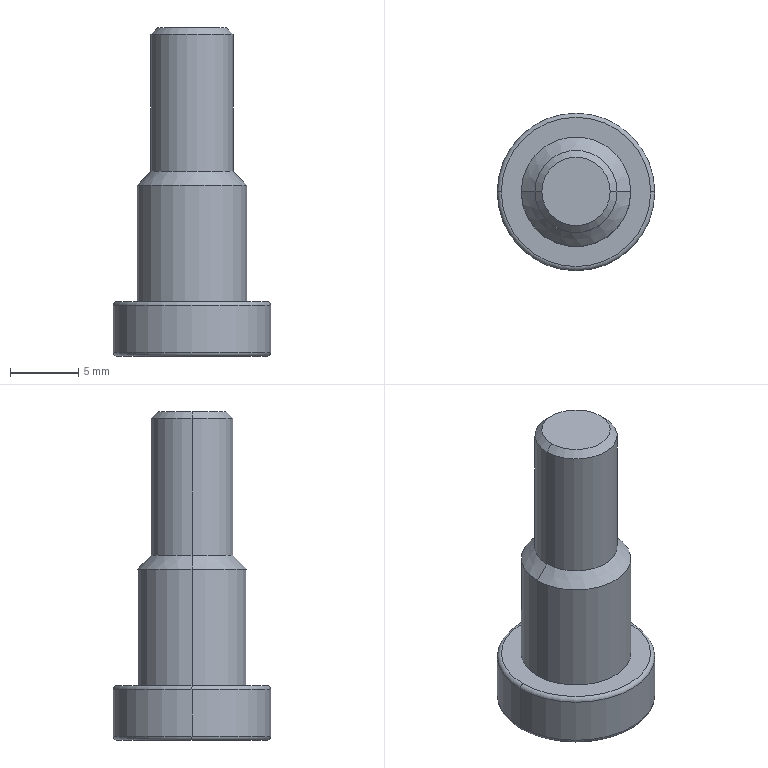Part | 1 solid | 26 faces | box 11.5 x 11.5 x 24 mm | volume 1109 mm3 | plane 10 | cone 6 | cylinder 6 | torus 4 | commonest cylinder face diameters 6 x2 8 x2 11.5 x2
STEP:
#1=CARTESIAN_POINT('',(-5.45,0.,0.));
#2=VERTEX_POINT('',#1);
#3=CARTESIAN_POINT('',(5.45,0.,0.));
#4=VERTEX_POINT('',#3);
#5=CARTESIAN_POINT('',(0.,0.,0.));
#6=DIRECTION('',(0.,0.,-1.));
#7=DIRECTION('',(1.,0.,0.));
#8=AXIS2_PLACEMENT_3D('',#5,#6,#7);
#9=CIRCLE('',#8,5.45);
#10=EDGE_CURVE('',#2,#4,#9,.T.);
#11=ORIENTED_EDGE('',*,*,#10,.F.);
#12=CARTESIAN_POINT('',(-5.75,0.,0.3));
#13=VERTEX_POINT('',#12);
#14=CARTESIAN_POINT('',(-5.45,0.,0.3));
#15=DIRECTION('',(0.,1.,0.));
#16=DIRECTION('',(-1.,0.,0.));
#17=AXIS2_PLACEMENT_3D('',#14,#15,#16);
#18=CIRCLE('',#17,0.3);
#19=EDGE_CURVE('',#2,#13,#18,.T.);
#20=ORIENTED_EDGE('',*,*,#19,.T.);
#21=CARTESIAN_POINT('',(5.75,0.,0.3));
#22=VERTEX_POINT('',#21);
#23=CARTESIAN_POINT('',(0.,0.,0.3));
#24=DIRECTION('',(0.,0.,1.));
#25=DIRECTION('',(1.,0.,0.));
#26=AXIS2_PLACEMENT_3D('',#23,#24,#25);
#27=CIRCLE('',#26,5.75);
#28=EDGE_CURVE('',#22,#13,#27,.T.);
#29=ORIENTED_EDGE('',*,*,#28,.F.);
#30=CARTESIAN_POINT('',(5.45,0.,0.3));
#31=DIRECTION('',(0.,-1.,0.));
#32=DIRECTION('',(0.,0.,-1.));
#33=AXIS2_PLACEMENT_3D('',#30,#31,#32);
#34=CIRCLE('',#33,0.3);
#35=EDGE_CURVE('',#4,#22,#34,.T.);
#36=ORIENTED_EDGE('',*,*,#35,.F.);
#37=EDGE_LOOP('',(#11,#20,#29,#36));
#38=FACE_OUTER_BOUND('',#37,.T.);
#39=CARTESIAN_POINT('',(0.,0.,0.3));
#40=DIRECTION('',(0.,0.,1.));
#41=DIRECTION('',(1.,0.,0.));
#42=AXIS2_PLACEMENT_3D('',#39,#40,#41);
#43=TOROIDAL_SURFACE('',#42,5.45,0.3);
#44=ADVANCED_FACE('',(#38),#43,.T.);
#45=CARTESIAN_POINT('',(-5.75,0.,3.7));
#46=VERTEX_POINT('',#45);
#47=CARTESIAN_POINT('',(5.75,0.,3.7));
#48=VERTEX_POINT('',#47);
#49=CARTESIAN_POINT('',(0.,0.,3.7));
#50=DIRECTION('',(0.,0.,-1.));
#51=DIRECTION('',(1.,0.,0.));
#52=AXIS2_PLACEMENT_3D('',#49,#50,#51);
#53=CIRCLE('',#52,5.75);
#54=EDGE_CURVE('',#46,#48,#53,.T.);
#55=ORIENTED_EDGE('',*,*,#54,.F.);
#56=CARTESIAN_POINT('',(-5.45,0.,4.));
#57=VERTEX_POINT('',#56);
#58=CARTESIAN_POINT('',(-5.45,0.,3.7));
#59=DIRECTION('',(0.,1.,0.));
#60=DIRECTION('',(-1.,0.,0.));
#61=AXIS2_PLACEMENT_3D('',#58,#59,#60);
#62=CIRCLE('',#61,0.3);
#63=EDGE_CURVE('',#46,#57,#62,.T.);
#64=ORIENTED_EDGE('',*,*,#63,.T.);
#65=CARTESIAN_POINT('',(5.45,0.,4.));
#66=VERTEX_POINT('',#65);
#67=CARTESIAN_POINT('',(0.,0.,4.));
#68=DIRECTION('',(0.,0.,1.));
#69=DIRECTION('',(1.,0.,0.));
#70=AXIS2_PLACEMENT_3D('',#67,#68,#69);
#71=CIRCLE('',#70,5.45);
#72=EDGE_CURVE('',#66,#57,#71,.T.);
#73=ORIENTED_EDGE('',*,*,#72,.F.);
#74=CARTESIAN_POINT('',(5.45,0.,3.7));
#75=DIRECTION('',(0.,-1.,0.));
#76=DIRECTION('',(0.,0.,-1.));
#77=AXIS2_PLACEMENT_3D('',#74,#75,#76);
#78=CIRCLE('',#77,0.3);
#79=EDGE_CURVE('',#48,#66,#78,.T.);
#80=ORIENTED_EDGE('',*,*,#79,.F.);
#81=EDGE_LOOP('',(#55,#64,#73,#80));
#82=FACE_OUTER_BOUND('',#81,.T.);
#83=CARTESIAN_POINT('',(0.,0.,3.7));
#84=DIRECTION('',(0.,0.,1.));
#85=DIRECTION('',(1.,0.,0.));
#86=AXIS2_PLACEMENT_3D('',#83,#84,#85);
#87=TOROIDAL_SURFACE('',#86,5.45,0.3);
#88=ADVANCED_FACE('',(#82),#87,.T.);
#89=CARTESIAN_POINT('',(2.887,0.,0.01325));
#90=VERTEX_POINT('',#89);
#91=CARTESIAN_POINT('',(1.443,-2.5,0.01325));
#92=VERTEX_POINT('',#91);
#93=CARTESIAN_POINT('',(2.887,0.,0.01325));
#94=CARTESIAN_POINT('',(2.826,-0.1053,0.07405));
#95=CARTESIAN_POINT('',(2.737,-0.2595,0.1543));
#96=CARTESIAN_POINT('',(2.637,-0.4329,0.2287));
#97=CARTESIAN_POINT('',(2.588,-0.518,0.2612));
#98=CARTESIAN_POINT('',(2.567,-0.5541,0.274));
#99=CARTESIAN_POINT('',(2.553,-0.5781,0.2824));
#100=CARTESIAN_POINT('',(2.547,-0.5883,0.2859));
#101=CARTESIAN_POINT('',(2.413,-0.8207,0.3629));
#102=CARTESIAN_POINT('',(2.289,-1.035,0.3994));
#103=CARTESIAN_POINT('',(2.107,-1.35,0.4003));
#104=CARTESIAN_POINT('',(2.015,-1.51,0.3871));
#105=CARTESIAN_POINT('',(1.906,-1.699,0.3481));
#106=CARTESIAN_POINT('',(1.851,-1.794,0.3226));
#107=CARTESIAN_POINT('',(1.827,-1.835,0.3104));
#108=CARTESIAN_POINT('',(1.812,-1.862,0.302));
#109=CARTESIAN_POINT('',(1.803,-1.878,0.2971));
#110=CARTESIAN_POINT('',(1.684,-2.083,0.2301));
#111=CARTESIAN_POINT('',(1.567,-2.286,0.1368));
#112=CARTESIAN_POINT('',(1.443,-2.5,0.01325));
#113=B_SPLINE_CURVE_WITH_KNOTS('',3,(#93,#94,#95,#96,#97,#98,#99,#100,#101,#102,#103,#104,#105,#106,#107,#108,#109,#110,#111,#112),.UNSPECIFIED.,.F.,.F.,(4,1,1,1,2,2,2,1,1,1,2,2,4),(0.,0.125,0.1875,0.2187,0.2344,0.25,0.5,0.625,0.6875,0.7187,0.7344,0.75,1.),.UNSPECIFIED.);
#114=EDGE_CURVE('',#90,#92,#113,.T.);
#115=ORIENTED_EDGE('',*,*,#114,.F.);
#116=CARTESIAN_POINT('',(2.9,0.,0.));
#117=VERTEX_POINT('',#116);
#118=CARTESIAN_POINT('',(2.4,0.,0.5));
#119=DIRECTION('',(0.7071,0.,-0.7071));
#120=VECTOR('',#119,1000.);
#121=LINE('',#118,#120);
#122=EDGE_CURVE('',#90,#117,#121,.T.);
#123=ORIENTED_EDGE('',*,*,#122,.T.);
#124=CARTESIAN_POINT('',(-2.9,0.,0.));
#125=VERTEX_POINT('',#124);
#126=CARTESIAN_POINT('',(0.,0.,0.));
#127=DIRECTION('',(0.,0.,1.));
#128=DIRECTION('',(1.,0.,0.));
#129=AXIS2_PLACEMENT_3D('',#126,#127,#128);
#130=CIRCLE('',#129,2.9);
#131=EDGE_CURVE('',#125,#117,#130,.T.);
#132=ORIENTED_EDGE('',*,*,#131,.F.);
#133=CARTESIAN_POINT('',(-2.887,0.,0.01325));
#134=VERTEX_POINT('',#133);
#135=CARTESIAN_POINT('',(-2.4,0.,0.5));
#136=DIRECTION('',(-0.7071,0.,-0.7071));
#137=VECTOR('',#136,1000.);
#138=LINE('',#135,#137);
#139=EDGE_CURVE('',#134,#125,#138,.T.);
#140=ORIENTED_EDGE('',*,*,#139,.F.);
#141=CARTESIAN_POINT('',(-1.443,-2.5,0.01325));
#142=VERTEX_POINT('',#141);
#143=CARTESIAN_POINT('',(-1.443,-2.5,0.01325));
#144=CARTESIAN_POINT('',(-1.504,-2.395,0.07405));
#145=CARTESIAN_POINT('',(-1.593,-2.24,0.1543));
#146=CARTESIAN_POINT('',(-1.693,-2.067,0.2287));
#147=CARTESIAN_POINT('',(-1.742,-1.982,0.2612));
#148=CARTESIAN_POINT('',(-1.763,-1.946,0.274));
#149=CARTESIAN_POINT('',(-1.777,-1.922,0.2824));
#150=CARTESIAN_POINT('',(-1.783,-1.912,0.2859));
#151=CARTESIAN_POINT('',(-1.917,-1.679,0.3629));
#152=CARTESIAN_POINT('',(-2.041,-1.465,0.3994));
#153=CARTESIAN_POINT('',(-2.223,-1.15,0.4003));
#154=CARTESIAN_POINT('',(-2.315,-0.9904,0.3871));
#155=CARTESIAN_POINT('',(-2.424,-0.8014,0.3481));
#156=CARTESIAN_POINT('',(-2.479,-0.7061,0.3226));
#157=CARTESIAN_POINT('',(-2.503,-0.6651,0.3104));
#158=CARTESIAN_POINT('',(-2.519,-0.6377,0.302));
#159=CARTESIAN_POINT('',(-2.527,-0.6224,0.2971));
#160=CARTESIAN_POINT('',(-2.646,-0.4174,0.2301));
#161=CARTESIAN_POINT('',(-2.763,-0.214,0.1368));
#162=CARTESIAN_POINT('',(-2.887,0.,0.01325));
#163=B_SPLINE_CURVE_WITH_KNOTS('',3,(#143,#144,#145,#146,#147,#148,#149,#150,#151,#152,#153,#154,#155,#156,#157,#158,#159,#160,#161,#162),.UNSPECIFIED.,.F.,.F.,(4,1,1,1,2,2,2,1,1,1,2,2,4),(0.,0.125,0.1875,0.2188,0.2344,0.25,0.5,0.625,0.6875,0.7187,0.7344,0.75,1.),.UNSPECIFIED.);
#164=EDGE_CURVE('',#142,#134,#163,.T.);
#165=ORIENTED_EDGE('',*,*,#164,.F.);
#166=CARTESIAN_POINT('',(1.443,-2.5,0.01325));
#167=CARTESIAN_POINT('',(1.321,-2.5,0.0745));
#168=CARTESIAN_POINT('',(1.142,-2.5,0.1553));
#169=CARTESIAN_POINT('',(0.9399,-2.5,0.23));
#170=CARTESIAN_POINT('',(0.841,-2.5,0.2626));
#171=CARTESIAN_POINT('',(0.799,-2.5,0.2754));
#172=CARTESIAN_POINT('',(0.7711,-2.5,0.2838));
#173=CARTESIAN_POINT('',(0.7591,-2.5,0.2873));
#174=CARTESIAN_POINT('',(0.4909,-2.5,0.3638));
#175=CARTESIAN_POINT('',(0.2428,-2.5,0.3999));
#176=CARTESIAN_POINT('',(-0.1205,-2.5,0.4001));
#177=CARTESIAN_POINT('',(-0.3043,-2.5,0.3866));
#178=CARTESIAN_POINT('',(-0.5223,-2.5,0.3472));
#179=CARTESIAN_POINT('',(-0.6323,-2.5,0.3215));
#180=CARTESIAN_POINT('',(-0.6796,-2.5,0.3093));
#181=CARTESIAN_POINT('',(-0.7112,-2.5,0.3008));
#182=CARTESIAN_POINT('',(-0.729,-2.5,0.2959));
#183=CARTESIAN_POINT('',(-0.9643,-2.5,0.2289));
#184=CARTESIAN_POINT('',(-1.198,-2.5,0.136));
#185=CARTESIAN_POINT('',(-1.443,-2.5,0.01325));
#186=B_SPLINE_CURVE_WITH_KNOTS('',3,(#166,#167,#168,#169,#170,#171,#172,#173,#174,#175,#176,#177,#178,#179,#180,#181,#182,#183,#184,#185),.UNSPECIFIED.,.F.,.F.,(4,1,1,1,2,2,2,1,1,1,2,2,4),(0.,0.125,0.1875,0.2187,0.2344,0.25,0.5,0.625,0.6875,0.7187,0.7344,0.75,1.),.UNSPECIFIED.);
#187=EDGE_CURVE('',#92,#142,#186,.T.);
#188=ORIENTED_EDGE('',*,*,#187,.F.);
#189=EDGE_LOOP('',(#115,#123,#132,#140,#165,#188));
#190=FACE_OUTER_BOUND('',#189,.T.);
#191=CARTESIAN_POINT('',(0.,0.,0.5));
#192=DIRECTION('',(0.,0.,-1.));
#193=DIRECTION('',(-1.,0.,0.));
#194=AXIS2_PLACEMENT_3D('',#191,#192,#193);
#195=CONICAL_SURFACE('',#194,2.4,0.7854);
#196=ADVANCED_FACE('',(#190),#195,.F.);
#197=CARTESIAN_POINT('',(2.5,0.,24.));
#198=VERTEX_POINT('',#197);
#199=CARTESIAN_POINT('',(-2.5,0.,24.));
#200=VERTEX_POINT('',#199);
#201=CARTESIAN_POINT('',(0.,0.,24.));
#202=DIRECTION('',(0.,0.,1.));
#203=DIRECTION('',(1.,0.,0.));
#204=AXIS2_PLACEMENT_3D('',#201,#202,#203);
#205=CIRCLE('',#204,2.5);
#206=EDGE_CURVE('',#198,#200,#205,.T.);
#207=ORIENTED_EDGE('',*,*,#206,.F.);
#208=CARTESIAN_POINT('',(3.,0.,23.5));
#209=VERTEX_POINT('',#208);
#210=CARTESIAN_POINT('',(2.5,0.,24.));
#211=DIRECTION('',(0.7071,0.,-0.7071));
#212=VECTOR('',#211,1000.);
#213=LINE('',#210,#212);
#214=EDGE_CURVE('',#198,#209,#213,.T.);
#215=ORIENTED_EDGE('',*,*,#214,.T.);
#216=CARTESIAN_POINT('',(-3.,0.,23.5));
#217=VERTEX_POINT('',#216);
#218=CARTESIAN_POINT('',(0.,0.,23.5));
#219=DIRECTION('',(0.,0.,-1.));
#220=DIRECTION('',(1.,0.,0.));
#221=AXIS2_PLACEMENT_3D('',#218,#219,#220);
#222=CIRCLE('',#221,3.);
#223=EDGE_CURVE('',#217,#209,#222,.T.);
#224=ORIENTED_EDGE('',*,*,#223,.F.);
#225=CARTESIAN_POINT('',(-2.5,0.,24.));
#226=DIRECTION('',(-0.7071,0.,-0.7071));
#227=VECTOR('',#226,1000.);
#228=LINE('',#225,#227);
#229=EDGE_CURVE('',#200,#217,#228,.T.);
#230=ORIENTED_EDGE('',*,*,#229,.F.);
#231=EDGE_LOOP('',(#207,#215,#224,#230));
#232=FACE_OUTER_BOUND('',#231,.T.);
#233=CARTESIAN_POINT('',(0.,0.,24.));
#234=DIRECTION('',(0.,0.,-1.));
#235=DIRECTION('',(-1.,0.,0.));
#236=AXIS2_PLACEMENT_3D('',#233,#234,#235);
#237=CONICAL_SURFACE('',#236,2.5,0.7854);
#238=ADVANCED_FACE('',(#232),#237,.T.);
#239=CARTESIAN_POINT('',(3.,0.,13.5));
#240=VERTEX_POINT('',#239);
#241=CARTESIAN_POINT('',(-3.,0.,13.5));
#242=VERTEX_POINT('',#241);
#243=CARTESIAN_POINT('',(0.,0.,13.5));
#244=DIRECTION('',(0.,0.,1.));
#245=DIRECTION('',(1.,0.,0.));
#246=AXIS2_PLACEMENT_3D('',#243,#244,#245);
#247=CIRCLE('',#246,3.);
#248=EDGE_CURVE('',#240,#242,#247,.T.);
#249=ORIENTED_EDGE('',*,*,#248,.F.);
#250=CARTESIAN_POINT('',(4.,0.,12.5));
#251=VERTEX_POINT('',#250);
#252=CARTESIAN_POINT('',(3.,0.,13.5));
#253=DIRECTION('',(0.7071,0.,-0.7071));
#254=VECTOR('',#253,1000.);
#255=LINE('',#252,#254);
#256=EDGE_CURVE('',#240,#251,#255,.T.);
#257=ORIENTED_EDGE('',*,*,#256,.T.);
#258=CARTESIAN_POINT('',(-4.,0.,12.5));
#259=VERTEX_POINT('',#258);
#260=CARTESIAN_POINT('',(0.,0.,12.5));
#261=DIRECTION('',(0.,0.,-1.));
#262=DIRECTION('',(1.,0.,0.));
#263=AXIS2_PLACEMENT_3D('',#260,#261,#262);
#264=CIRCLE('',#263,4.);
#265=EDGE_CURVE('',#259,#251,#264,.T.);
#266=ORIENTED_EDGE('',*,*,#265,.F.);
#267=CARTESIAN_POINT('',(-3.,0.,13.5));
#268=DIRECTION('',(-0.7071,0.,-0.7071));
#269=VECTOR('',#268,1000.);
#270=LINE('',#267,#269);
#271=EDGE_CURVE('',#242,#259,#270,.T.);
#272=ORIENTED_EDGE('',*,*,#271,.F.);
#273=EDGE_LOOP('',(#249,#257,#266,#272));
#274=FACE_OUTER_BOUND('',#273,.T.);
#275=CARTESIAN_POINT('',(0.,0.,13.5));
#276=DIRECTION('',(0.,0.,-1.));
#277=DIRECTION('',(-1.,0.,0.));
#278=AXIS2_PLACEMENT_3D('',#275,#276,#277);
#279=CONICAL_SURFACE('',#278,3.,0.7854);
#280=ADVANCED_FACE('',(#274),#279,.T.);
#281=ORIENTED_EDGE('',*,*,#223,.T.);
#282=CARTESIAN_POINT('',(3.,0.,24.));
#283=DIRECTION('',(0.,0.,-1.));
#284=VECTOR('',#283,1000.);
#285=LINE('',#282,#284);
#286=EDGE_CURVE('',#209,#240,#285,.T.);
#287=ORIENTED_EDGE('',*,*,#286,.T.);
#288=ORIENTED_EDGE('',*,*,#248,.T.);
#289=CARTESIAN_POINT('',(-3.,0.,24.));
#290=DIRECTION('',(0.,0.,-1.));
#291=VECTOR('',#290,1000.);
#292=LINE('',#289,#291);
#293=EDGE_CURVE('',#217,#242,#292,.T.);
#294=ORIENTED_EDGE('',*,*,#293,.F.);
#295=EDGE_LOOP('',(#281,#287,#288,#294));
#296=FACE_OUTER_BOUND('',#295,.T.);
#297=CARTESIAN_POINT('',(0.,0.,24.));
#298=DIRECTION('',(0.,0.,-1.));
#299=DIRECTION('',(-1.,0.,0.));
#300=AXIS2_PLACEMENT_3D('',#297,#298,#299);
#301=CYLINDRICAL_SURFACE('',#300,3.);
#302=ADVANCED_FACE('',(#296),#301,.T.);
#303=ORIENTED_EDGE('',*,*,#265,.T.);
#304=CARTESIAN_POINT('',(4.,0.,4.));
#305=VERTEX_POINT('',#304);
#306=CARTESIAN_POINT('',(4.,0.,13.5));
#307=DIRECTION('',(0.,0.,-1.));
#308=VECTOR('',#307,1000.);
#309=LINE('',#306,#308);
#310=EDGE_CURVE('',#251,#305,#309,.T.);
#311=ORIENTED_EDGE('',*,*,#310,.T.);
#312=CARTESIAN_POINT('',(-4.,0.,4.));
#313=VERTEX_POINT('',#312);
#314=CARTESIAN_POINT('',(0.,0.,4.));
#315=DIRECTION('',(0.,0.,1.));
#316=DIRECTION('',(1.,0.,0.));
#317=AXIS2_PLACEMENT_3D('',#314,#315,#316);
#318=CIRCLE('',#317,4.);
#319=EDGE_CURVE('',#305,#313,#318,.T.);
#320=ORIENTED_EDGE('',*,*,#319,.T.);
#321=CARTESIAN_POINT('',(-4.,0.,13.5));
#322=DIRECTION('',(0.,0.,-1.));
#323=VECTOR('',#322,1000.);
#324=LINE('',#321,#323);
#325=EDGE_CURVE('',#259,#313,#324,.T.);
#326=ORIENTED_EDGE('',*,*,#325,.F.);
#327=EDGE_LOOP('',(#303,#311,#320,#326));
#328=FACE_OUTER_BOUND('',#327,.T.);
#329=CARTESIAN_POINT('',(0.,0.,13.5));
#330=DIRECTION('',(0.,0.,-1.));
#331=DIRECTION('',(-1.,0.,0.));
#332=AXIS2_PLACEMENT_3D('',#329,#330,#331);
#333=CYLINDRICAL_SURFACE('',#332,4.);
#334=ADVANCED_FACE('',(#328),#333,.T.);
#335=ORIENTED_EDGE('',*,*,#54,.T.);
#336=CARTESIAN_POINT('',(5.75,0.,4.));
#337=DIRECTION('',(0.,0.,-1.));
#338=VECTOR('',#337,1000.);
#339=LINE('',#336,#338);
#340=EDGE_CURVE('',#48,#22,#339,.T.);
#341=ORIENTED_EDGE('',*,*,#340,.T.);
#342=ORIENTED_EDGE('',*,*,#28,.T.);
#343=CARTESIAN_POINT('',(-5.75,0.,4.));
#344=DIRECTION('',(0.,0.,-1.));
#345=VECTOR('',#344,1000.);
#346=LINE('',#343,#345);
#347=EDGE_CURVE('',#46,#13,#346,.T.);
#348=ORIENTED_EDGE('',*,*,#347,.F.);
#349=EDGE_LOOP('',(#335,#341,#342,#348));
#350=FACE_OUTER_BOUND('',#349,.T.);
#351=CARTESIAN_POINT('',(0.,0.,4.));
#352=DIRECTION('',(0.,0.,-1.));
#353=DIRECTION('',(-1.,0.,0.));
#354=AXIS2_PLACEMENT_3D('',#351,#352,#353);
#355=CYLINDRICAL_SURFACE('',#354,5.75);
#356=ADVANCED_FACE('',(#350),#355,.T.);
#357=ORIENTED_EDGE('',*,*,#340,.F.);
#358=CARTESIAN_POINT('',(0.,0.,3.7));
#359=DIRECTION('',(0.,0.,-1.));
#360=DIRECTION('',(1.,0.,0.));
#361=AXIS2_PLACEMENT_3D('',#358,#359,#360);
#362=CIRCLE('',#361,5.75);
#363=EDGE_CURVE('',#48,#46,#362,.T.);
#364=ORIENTED_EDGE('',*,*,#363,.T.);
#365=ORIENTED_EDGE('',*,*,#347,.T.);
#366=CARTESIAN_POINT('',(0.,0.,0.3));
#367=DIRECTION('',(0.,0.,1.));
#368=DIRECTION('',(1.,0.,0.));
#369=AXIS2_PLACEMENT_3D('',#366,#367,#368);
#370=CIRCLE('',#369,5.75);
#371=EDGE_CURVE('',#13,#22,#370,.T.);
#372=ORIENTED_EDGE('',*,*,#371,.T.);
#373=EDGE_LOOP('',(#357,#364,#365,#372));
#374=FACE_OUTER_BOUND('',#373,.T.);
#375=CARTESIAN_POINT('',(0.,0.,4.));
#376=DIRECTION('',(0.,0.,-1.));
#377=DIRECTION('',(-1.,0.,0.));
#378=AXIS2_PLACEMENT_3D('',#375,#376,#377);
#379=CYLINDRICAL_SURFACE('',#378,5.75);
#380=ADVANCED_FACE('',(#374),#379,.T.);
#381=ORIENTED_EDGE('',*,*,#72,.T.);
#382=CARTESIAN_POINT('',(0.,0.,4.));
#383=DIRECTION('',(0.,0.,1.));
#384=DIRECTION('',(1.,0.,0.));
#385=AXIS2_PLACEMENT_3D('',#382,#383,#384);
#386=CIRCLE('',#385,5.45);
#387=EDGE_CURVE('',#57,#66,#386,.T.);
#388=ORIENTED_EDGE('',*,*,#387,.T.);
#389=EDGE_LOOP('',(#381,#388));
#390=FACE_OUTER_BOUND('',#389,.T.);
#391=CARTESIAN_POINT('',(0.,0.,4.));
#392=DIRECTION('',(0.,0.,1.));
#393=DIRECTION('',(1.,0.,0.));
#394=AXIS2_PLACEMENT_3D('',#391,#392,#393);
#395=CIRCLE('',#394,4.);
#396=EDGE_CURVE('',#313,#305,#395,.T.);
#397=ORIENTED_EDGE('',*,*,#396,.F.);
#398=ORIENTED_EDGE('',*,*,#319,.F.);
#399=EDGE_LOOP('',(#397,#398));
#400=FACE_BOUND('',#399,.T.);
#401=CARTESIAN_POINT('',(0.,0.,4.));
#402=DIRECTION('',(0.,0.,1.));
#403=DIRECTION('',(1.,0.,0.));
#404=AXIS2_PLACEMENT_3D('',#401,#402,#403);
#405=PLANE('',#404);
#406=ADVANCED_FACE('',(#390,#400),#405,.T.);
#407=CARTESIAN_POINT('',(0.,0.,0.));
#408=DIRECTION('',(0.,0.,-1.));
#409=DIRECTION('',(1.,0.,0.));
#410=AXIS2_PLACEMENT_3D('',#407,#408,#409);
#411=CIRCLE('',#410,5.45);
#412=EDGE_CURVE('',#4,#2,#411,.T.);
#413=ORIENTED_EDGE('',*,*,#412,.T.);
#414=ORIENTED_EDGE('',*,*,#10,.T.);
#415=EDGE_LOOP('',(#413,#414));
#416=FACE_OUTER_BOUND('',#415,.T.);
#417=ORIENTED_EDGE('',*,*,#131,.T.);
#418=CARTESIAN_POINT('',(0.,0.,0.));
#419=DIRECTION('',(0.,0.,1.));
#420=DIRECTION('',(1.,0.,0.));
#421=AXIS2_PLACEMENT_3D('',#418,#419,#420);
#422=CIRCLE('',#421,2.9);
#423=EDGE_CURVE('',#117,#125,#422,.T.);
#424=ORIENTED_EDGE('',*,*,#423,.T.);
#425=EDGE_LOOP('',(#417,#424));
#426=FACE_BOUND('',#425,.T.);
#427=CARTESIAN_POINT('',(0.,0.,0.));
#428=DIRECTION('',(0.,0.,1.));
#429=DIRECTION('',(1.,0.,0.));
#430=AXIS2_PLACEMENT_3D('',#427,#428,#429);
#431=PLANE('',#430);
#432=ADVANCED_FACE('',(#416,#426),#431,.F.);
#433=ORIENTED_EDGE('',*,*,#310,.F.);
#434=CARTESIAN_POINT('',(0.,0.,12.5));
#435=DIRECTION('',(0.,0.,-1.));
#436=DIRECTION('',(1.,0.,0.));
#437=AXIS2_PLACEMENT_3D('',#434,#435,#436);
#438=CIRCLE('',#437,4.);
#439=EDGE_CURVE('',#251,#259,#438,.T.);
#440=ORIENTED_EDGE('',*,*,#439,.T.);
#441=ORIENTED_EDGE('',*,*,#325,.T.);
#442=ORIENTED_EDGE('',*,*,#396,.T.);
#443=EDGE_LOOP('',(#433,#440,#441,#442));
#444=FACE_OUTER_BOUND('',#443,.T.);
#445=CARTESIAN_POINT('',(0.,0.,13.5));
#446=DIRECTION('',(0.,0.,-1.));
#447=DIRECTION('',(-1.,0.,0.));
#448=AXIS2_PLACEMENT_3D('',#445,#446,#447);
#449=CYLINDRICAL_SURFACE('',#448,4.);
#450=ADVANCED_FACE('',(#444),#449,.T.);
#451=ORIENTED_EDGE('',*,*,#286,.F.);
#452=CARTESIAN_POINT('',(0.,0.,23.5));
#453=DIRECTION('',(0.,0.,-1.));
#454=DIRECTION('',(1.,0.,0.));
#455=AXIS2_PLACEMENT_3D('',#452,#453,#454);
#456=CIRCLE('',#455,3.);
#457=EDGE_CURVE('',#209,#217,#456,.T.);
#458=ORIENTED_EDGE('',*,*,#457,.T.);
#459=ORIENTED_EDGE('',*,*,#293,.T.);
#460=CARTESIAN_POINT('',(0.,0.,13.5));
#461=DIRECTION('',(0.,0.,1.));
#462=DIRECTION('',(1.,0.,0.));
#463=AXIS2_PLACEMENT_3D('',#460,#461,#462);
#464=CIRCLE('',#463,3.);
#465=EDGE_CURVE('',#242,#240,#464,.T.);
#466=ORIENTED_EDGE('',*,*,#465,.T.);
#467=EDGE_LOOP('',(#451,#458,#459,#466));
#468=FACE_OUTER_BOUND('',#467,.T.);
#469=CARTESIAN_POINT('',(0.,0.,24.));
#470=DIRECTION('',(0.,0.,-1.));
#471=DIRECTION('',(-1.,0.,0.));
#472=AXIS2_PLACEMENT_3D('',#469,#470,#471);
#473=CYLINDRICAL_SURFACE('',#472,3.);
#474=ADVANCED_FACE('',(#468),#473,.T.);
#475=CARTESIAN_POINT('',(0.,0.,24.));
#476=DIRECTION('',(0.,0.,1.));
#477=DIRECTION('',(1.,0.,0.));
#478=AXIS2_PLACEMENT_3D('',#475,#476,#477);
#479=CIRCLE('',#478,2.5);
#480=EDGE_CURVE('',#200,#198,#479,.T.);
#481=ORIENTED_EDGE('',*,*,#480,.T.);
#482=ORIENTED_EDGE('',*,*,#206,.T.);
#483=EDGE_LOOP('',(#481,#482));
#484=FACE_OUTER_BOUND('',#483,.T.);
#485=CARTESIAN_POINT('',(0.,0.,24.));
#486=DIRECTION('',(0.,0.,1.));
#487=DIRECTION('',(1.,0.,0.));
#488=AXIS2_PLACEMENT_3D('',#485,#486,#487);
#489=PLANE('',#488);
#490=ADVANCED_FACE('',(#484),#489,.T.);
#491=ORIENTED_EDGE('',*,*,#256,.F.);
#492=ORIENTED_EDGE('',*,*,#465,.F.);
#493=ORIENTED_EDGE('',*,*,#271,.T.);
#494=ORIENTED_EDGE('',*,*,#439,.F.);
#495=EDGE_LOOP('',(#491,#492,#493,#494));
#496=FACE_OUTER_BOUND('',#495,.T.);
#497=CARTESIAN_POINT('',(0.,0.,13.5));
#498=DIRECTION('',(0.,0.,-1.));
#499=DIRECTION('',(-1.,0.,0.));
#500=AXIS2_PLACEMENT_3D('',#497,#498,#499);
#501=CONICAL_SURFACE('',#500,3.,0.7854);
#502=ADVANCED_FACE('',(#496),#501,.T.);
#503=ORIENTED_EDGE('',*,*,#214,.F.);
#504=ORIENTED_EDGE('',*,*,#480,.F.);
#505=ORIENTED_EDGE('',*,*,#229,.T.);
#506=ORIENTED_EDGE('',*,*,#457,.F.);
#507=EDGE_LOOP('',(#503,#504,#505,#506));
#508=FACE_OUTER_BOUND('',#507,.T.);
#509=CARTESIAN_POINT('',(0.,0.,24.));
#510=DIRECTION('',(0.,0.,-1.));
#511=DIRECTION('',(-1.,0.,0.));
#512=AXIS2_PLACEMENT_3D('',#509,#510,#511);
#513=CONICAL_SURFACE('',#512,2.5,0.7854);
#514=ADVANCED_FACE('',(#508),#513,.T.);
#515=ORIENTED_EDGE('',*,*,#122,.F.);
#516=CARTESIAN_POINT('',(1.443,2.5,0.01325));
#517=VERTEX_POINT('',#516);
#518=CARTESIAN_POINT('',(1.443,2.5,0.01325));
#519=CARTESIAN_POINT('',(1.504,2.395,0.07405));
#520=CARTESIAN_POINT('',(1.593,2.24,0.1543));
#521=CARTESIAN_POINT('',(1.693,2.067,0.2287));
#522=CARTESIAN_POINT('',(1.742,1.982,0.2612));
#523=CARTESIAN_POINT('',(1.763,1.946,0.274));
#524=CARTESIAN_POINT('',(1.777,1.922,0.2824));
#525=CARTESIAN_POINT('',(1.783,1.912,0.2859));
#526=CARTESIAN_POINT('',(1.917,1.679,0.3629));
#527=CARTESIAN_POINT('',(2.041,1.465,0.3994));
#528=CARTESIAN_POINT('',(2.223,1.15,0.4003));
#529=CARTESIAN_POINT('',(2.315,0.9904,0.3871));
#530=CARTESIAN_POINT('',(2.424,0.8014,0.3481));
#531=CARTESIAN_POINT('',(2.479,0.7061,0.3226));
#532=CARTESIAN_POINT('',(2.503,0.6651,0.3104));
#533=CARTESIAN_POINT('',(2.519,0.6377,0.302));
#534=CARTESIAN_POINT('',(2.527,0.6224,0.2971));
#535=CARTESIAN_POINT('',(2.646,0.4174,0.2301));
#536=CARTESIAN_POINT('',(2.763,0.214,0.1368));
#537=CARTESIAN_POINT('',(2.887,0.,0.01325));
#538=B_SPLINE_CURVE_WITH_KNOTS('',3,(#518,#519,#520,#521,#522,#523,#524,#525,#526,#527,#528,#529,#530,#531,#532,#533,#534,#535,#536,#537),.UNSPECIFIED.,.F.,.F.,(4,1,1,1,2,2,2,1,1,1,2,2,4),(0.,0.125,0.1875,0.2187,0.2344,0.25,0.5,0.625,0.6875,0.7188,0.7344,0.75,1.),.UNSPECIFIED.);
#539=EDGE_CURVE('',#517,#90,#538,.T.);
#540=ORIENTED_EDGE('',*,*,#539,.F.);
#541=CARTESIAN_POINT('',(-1.443,2.5,0.01325));
#542=VERTEX_POINT('',#541);
#543=CARTESIAN_POINT('',(-1.443,2.5,0.01325));
#544=CARTESIAN_POINT('',(-1.321,2.5,0.07454));
#545=CARTESIAN_POINT('',(-1.141,2.5,0.1553));
#546=CARTESIAN_POINT('',(-0.9395,2.5,0.2301));
#547=CARTESIAN_POINT('',(-0.8406,2.5,0.2627));
#548=CARTESIAN_POINT('',(-0.7986,2.5,0.2756));
#549=CARTESIAN_POINT('',(-0.7706,2.5,0.2839));
#550=CARTESIAN_POINT('',(-0.7587,2.5,0.2875));
#551=CARTESIAN_POINT('',(-0.4902,2.5,0.364));
#552=CARTESIAN_POINT('',(-0.2414,2.5,0.4));
#553=CARTESIAN_POINT('',(0.1216,2.5,0.4));
#554=CARTESIAN_POINT('',(0.3052,2.5,0.3865));
#555=CARTESIAN_POINT('',(0.523,2.5,0.347));
#556=CARTESIAN_POINT('',(0.6329,2.5,0.3214));
#557=CARTESIAN_POINT('',(0.6801,2.5,0.3092));
#558=CARTESIAN_POINT('',(0.7117,2.5,0.3007));
#559=CARTESIAN_POINT('',(0.7295,2.5,0.2958));
#560=CARTESIAN_POINT('',(0.9647,2.5,0.2288));
#561=CARTESIAN_POINT('',(1.198,2.5,0.1359));
#562=CARTESIAN_POINT('',(1.443,2.5,0.01325));
#563=B_SPLINE_CURVE_WITH_KNOTS('',3,(#543,#544,#545,#546,#547,#548,#549,#550,#551,#552,#553,#554,#555,#556,#557,#558,#559,#560,#561,#562),.UNSPECIFIED.,.F.,.F.,(4,1,1,1,2,2,2,1,1,1,2,2,4),(0.,0.125,0.1875,0.2188,0.2344,0.25,0.5,0.625,0.6875,0.7188,0.7344,0.75,1.),.UNSPECIFIED.);
#564=EDGE_CURVE('',#542,#517,#563,.T.);
#565=ORIENTED_EDGE('',*,*,#564,.F.);
#566=CARTESIAN_POINT('',(-2.887,0.,0.01325));
#567=CARTESIAN_POINT('',(-2.826,0.1053,0.07405));
#568=CARTESIAN_POINT('',(-2.737,0.2595,0.1543));
#569=CARTESIAN_POINT('',(-2.637,0.4329,0.2287));
#570=CARTESIAN_POINT('',(-2.588,0.518,0.2612));
#571=CARTESIAN_POINT('',(-2.567,0.5541,0.274));
#572=CARTESIAN_POINT('',(-2.553,0.5781,0.2824));
#573=CARTESIAN_POINT('',(-2.547,0.5883,0.2859));
#574=CARTESIAN_POINT('',(-2.413,0.8207,0.3629));
#575=CARTESIAN_POINT('',(-2.289,1.035,0.3994));
#576=CARTESIAN_POINT('',(-2.107,1.35,0.4003));
#577=CARTESIAN_POINT('',(-2.015,1.51,0.3871));
#578=CARTESIAN_POINT('',(-1.906,1.699,0.3481));
#579=CARTESIAN_POINT('',(-1.851,1.794,0.3226));
#580=CARTESIAN_POINT('',(-1.827,1.835,0.3104));
#581=CARTESIAN_POINT('',(-1.812,1.862,0.302));
#582=CARTESIAN_POINT('',(-1.803,1.878,0.2971));
#583=CARTESIAN_POINT('',(-1.684,2.083,0.2301));
#584=CARTESIAN_POINT('',(-1.567,2.286,0.1368));
#585=CARTESIAN_POINT('',(-1.443,2.5,0.01325));
#586=B_SPLINE_CURVE_WITH_KNOTS('',3,(#566,#567,#568,#569,#570,#571,#572,#573,#574,#575,#576,#577,#578,#579,#580,#581,#582,#583,#584,#585),.UNSPECIFIED.,.F.,.F.,(4,1,1,1,2,2,2,1,1,1,2,2,4),(0.,0.125,0.1875,0.2187,0.2344,0.25,0.5,0.625,0.6875,0.7187,0.7344,0.75,1.),.UNSPECIFIED.);
#587=EDGE_CURVE('',#134,#542,#586,.T.);
#588=ORIENTED_EDGE('',*,*,#587,.F.);
#589=ORIENTED_EDGE('',*,*,#139,.T.);
#590=ORIENTED_EDGE('',*,*,#423,.F.);
#591=EDGE_LOOP('',(#515,#540,#565,#588,#589,#590));
#592=FACE_OUTER_BOUND('',#591,.T.);
#593=CARTESIAN_POINT('',(0.,0.,0.5));
#594=DIRECTION('',(0.,0.,-1.));
#595=DIRECTION('',(-1.,0.,0.));
#596=AXIS2_PLACEMENT_3D('',#593,#594,#595);
#597=CONICAL_SURFACE('',#596,2.4,0.7854);
#598=ADVANCED_FACE('',(#592),#597,.F.);
#599=ORIENTED_EDGE('',*,*,#587,.T.);
#600=CARTESIAN_POINT('',(-1.443,2.5,3.));
#601=VERTEX_POINT('',#600);
#602=CARTESIAN_POINT('',(-1.443,2.5,3.));
#603=DIRECTION('',(0.,0.,-1.));
#604=VECTOR('',#603,1000.);
#605=LINE('',#602,#604);
#606=EDGE_CURVE('',#601,#542,#605,.T.);
#607=ORIENTED_EDGE('',*,*,#606,.F.);
#608=CARTESIAN_POINT('',(-2.887,0.,3.));
#609=VERTEX_POINT('',#608);
#610=CARTESIAN_POINT('',(-2.887,0.,3.));
#611=DIRECTION('',(0.5,0.866,0.));
#612=VECTOR('',#611,1000.);
#613=LINE('',#610,#612);
#614=EDGE_CURVE('',#609,#601,#613,.T.);
#615=ORIENTED_EDGE('',*,*,#614,.F.);
#616=CARTESIAN_POINT('',(-2.887,0.,3.));
#617=DIRECTION('',(0.,0.,-1.));
#618=VECTOR('',#617,1000.);
#619=LINE('',#616,#618);
#620=EDGE_CURVE('',#609,#134,#619,.T.);
#621=ORIENTED_EDGE('',*,*,#620,.T.);
#622=EDGE_LOOP('',(#599,#607,#615,#621));
#623=FACE_OUTER_BOUND('',#622,.T.);
#624=CARTESIAN_POINT('',(-2.887,0.,3.));
#625=DIRECTION('',(-0.866,0.5,0.));
#626=DIRECTION('',(0.,0.,1.));
#627=AXIS2_PLACEMENT_3D('',#624,#625,#626);
#628=PLANE('',#627);
#629=ADVANCED_FACE('',(#623),#628,.F.);
#630=ORIENTED_EDGE('',*,*,#164,.T.);
#631=ORIENTED_EDGE('',*,*,#620,.F.);
#632=CARTESIAN_POINT('',(-1.443,-2.5,3.));
#633=VERTEX_POINT('',#632);
#634=CARTESIAN_POINT('',(-1.443,-2.5,3.));
#635=DIRECTION('',(-0.5,0.866,0.));
#636=VECTOR('',#635,1000.);
#637=LINE('',#634,#636);
#638=EDGE_CURVE('',#633,#609,#637,.T.);
#639=ORIENTED_EDGE('',*,*,#638,.F.);
#640=CARTESIAN_POINT('',(-1.443,-2.5,3.));
#641=DIRECTION('',(0.,0.,-1.));
#642=VECTOR('',#641,1000.);
#643=LINE('',#640,#642);
#644=EDGE_CURVE('',#633,#142,#643,.T.);
#645=ORIENTED_EDGE('',*,*,#644,.T.);
#646=EDGE_LOOP('',(#630,#631,#639,#645));
#647=FACE_OUTER_BOUND('',#646,.T.);
#648=CARTESIAN_POINT('',(-1.443,-2.5,3.));
#649=DIRECTION('',(-0.866,-0.5,0.));
#650=DIRECTION('',(-0.5,0.866,0.));
#651=AXIS2_PLACEMENT_3D('',#648,#649,#650);
#652=PLANE('',#651);
#653=ADVANCED_FACE('',(#647),#652,.F.);
#654=ORIENTED_EDGE('',*,*,#187,.T.);
#655=ORIENTED_EDGE('',*,*,#644,.F.);
#656=CARTESIAN_POINT('',(1.443,-2.5,3.));
#657=VERTEX_POINT('',#656);
#658=CARTESIAN_POINT('',(1.443,-2.5,3.));
#659=DIRECTION('',(-1.,0.,0.));
#660=VECTOR('',#659,1000.);
#661=LINE('',#658,#660);
#662=EDGE_CURVE('',#657,#633,#661,.T.);
#663=ORIENTED_EDGE('',*,*,#662,.F.);
#664=CARTESIAN_POINT('',(1.443,-2.5,3.));
#665=DIRECTION('',(0.,0.,-1.));
#666=VECTOR('',#665,1000.);
#667=LINE('',#664,#666);
#668=EDGE_CURVE('',#657,#92,#667,.T.);
#669=ORIENTED_EDGE('',*,*,#668,.T.);
#670=EDGE_LOOP('',(#654,#655,#663,#669));
#671=FACE_OUTER_BOUND('',#670,.T.);
#672=CARTESIAN_POINT('',(1.443,-2.5,3.));
#673=DIRECTION('',(0.,-1.,0.));
#674=DIRECTION('',(0.,0.,-1.));
#675=AXIS2_PLACEMENT_3D('',#672,#673,#674);
#676=PLANE('',#675);
#677=ADVANCED_FACE('',(#671),#676,.F.);
#678=ORIENTED_EDGE('',*,*,#114,.T.);
#679=ORIENTED_EDGE('',*,*,#668,.F.);
#680=CARTESIAN_POINT('',(2.887,0.,3.));
#681=VERTEX_POINT('',#680);
#682=CARTESIAN_POINT('',(2.887,0.,3.));
#683=DIRECTION('',(-0.5,-0.866,0.));
#684=VECTOR('',#683,1000.);
#685=LINE('',#682,#684);
#686=EDGE_CURVE('',#681,#657,#685,.T.);
#687=ORIENTED_EDGE('',*,*,#686,.F.);
#688=CARTESIAN_POINT('',(2.887,0.,3.));
#689=DIRECTION('',(0.,0.,-1.));
#690=VECTOR('',#689,1000.);
#691=LINE('',#688,#690);
#692=EDGE_CURVE('',#681,#90,#691,.T.);
#693=ORIENTED_EDGE('',*,*,#692,.T.);
#694=EDGE_LOOP('',(#678,#679,#687,#693));
#695=FACE_OUTER_BOUND('',#694,.T.);
#696=CARTESIAN_POINT('',(2.887,0.,3.));
#697=DIRECTION('',(0.866,-0.5,0.));
#698=DIRECTION('',(0.,0.,-1.));
#699=AXIS2_PLACEMENT_3D('',#696,#697,#698);
#700=PLANE('',#699);
#701=ADVANCED_FACE('',(#695),#700,.F.);
#702=ORIENTED_EDGE('',*,*,#539,.T.);
#703=ORIENTED_EDGE('',*,*,#692,.F.);
#704=CARTESIAN_POINT('',(1.443,2.5,3.));
#705=VERTEX_POINT('',#704);
#706=CARTESIAN_POINT('',(1.443,2.5,3.));
#707=DIRECTION('',(0.5,-0.866,0.));
#708=VECTOR('',#707,1000.);
#709=LINE('',#706,#708);
#710=EDGE_CURVE('',#705,#681,#709,.T.);
#711=ORIENTED_EDGE('',*,*,#710,.F.);
#712=CARTESIAN_POINT('',(1.443,2.5,3.));
#713=DIRECTION('',(0.,0.,-1.));
#714=VECTOR('',#713,1000.);
#715=LINE('',#712,#714);
#716=EDGE_CURVE('',#705,#517,#715,.T.);
#717=ORIENTED_EDGE('',*,*,#716,.T.);
#718=EDGE_LOOP('',(#702,#703,#711,#717));
#719=FACE_OUTER_BOUND('',#718,.T.);
#720=CARTESIAN_POINT('',(1.443,2.5,3.));
#721=DIRECTION('',(0.866,0.5,0.));
#722=DIRECTION('',(0.,0.,-1.));
#723=AXIS2_PLACEMENT_3D('',#720,#721,#722);
#724=PLANE('',#723);
#725=ADVANCED_FACE('',(#719),#724,.F.);
#726=ORIENTED_EDGE('',*,*,#564,.T.);
#727=ORIENTED_EDGE('',*,*,#716,.F.);
#728=CARTESIAN_POINT('',(-1.443,2.5,3.));
#729=DIRECTION('',(1.,0.,0.));
#730=VECTOR('',#729,1000.);
#731=LINE('',#728,#730);
#732=EDGE_CURVE('',#601,#705,#731,.T.);
#733=ORIENTED_EDGE('',*,*,#732,.F.);
#734=ORIENTED_EDGE('',*,*,#606,.T.);
#735=EDGE_LOOP('',(#726,#727,#733,#734));
#736=FACE_OUTER_BOUND('',#735,.T.);
#737=CARTESIAN_POINT('',(-1.443,2.5,3.));
#738=DIRECTION('',(0.,1.,0.));
#739=DIRECTION('',(1.,0.,0.));
#740=AXIS2_PLACEMENT_3D('',#737,#738,#739);
#741=PLANE('',#740);
#742=ADVANCED_FACE('',(#736),#741,.F.);
#743=ORIENTED_EDGE('',*,*,#614,.T.);
#744=ORIENTED_EDGE('',*,*,#732,.T.);
#745=ORIENTED_EDGE('',*,*,#710,.T.);
#746=ORIENTED_EDGE('',*,*,#686,.T.);
#747=ORIENTED_EDGE('',*,*,#662,.T.);
#748=ORIENTED_EDGE('',*,*,#638,.T.);
#749=EDGE_LOOP('',(#743,#744,#745,#746,#747,#748));
#750=FACE_OUTER_BOUND('',#749,.T.);
#751=CARTESIAN_POINT('',(0.,0.,3.));
#752=DIRECTION('',(0.,0.,-1.));
#753=DIRECTION('',(0.,-1.,0.));
#754=AXIS2_PLACEMENT_3D('',#751,#752,#753);
#755=PLANE('',#754);
#756=ADVANCED_FACE('',(#750),#755,.T.);
#757=ORIENTED_EDGE('',*,*,#63,.F.);
#758=ORIENTED_EDGE('',*,*,#363,.F.);
#759=ORIENTED_EDGE('',*,*,#79,.T.);
#760=ORIENTED_EDGE('',*,*,#387,.F.);
#761=EDGE_LOOP('',(#757,#758,#759,#760));
#762=FACE_OUTER_BOUND('',#761,.T.);
#763=CARTESIAN_POINT('',(0.,0.,3.7));
#764=DIRECTION('',(0.,0.,1.));
#765=DIRECTION('',(1.,0.,0.));
#766=AXIS2_PLACEMENT_3D('',#763,#764,#765);
#767=TOROIDAL_SURFACE('',#766,5.45,0.3);
#768=ADVANCED_FACE('',(#762),#767,.T.);
#769=ORIENTED_EDGE('',*,*,#19,.F.);
#770=ORIENTED_EDGE('',*,*,#412,.F.);
#771=ORIENTED_EDGE('',*,*,#35,.T.);
#772=ORIENTED_EDGE('',*,*,#371,.F.);
#773=EDGE_LOOP('',(#769,#770,#771,#772));
#774=FACE_OUTER_BOUND('',#773,.T.);
#775=CARTESIAN_POINT('',(0.,0.,0.3));
#776=DIRECTION('',(0.,0.,1.));
#777=DIRECTION('',(1.,0.,0.));
#778=AXIS2_PLACEMENT_3D('',#775,#776,#777);
#779=TOROIDAL_SURFACE('',#778,5.45,0.3);
#780=ADVANCED_FACE('',(#774),#779,.T.);
#781=CLOSED_SHELL('',(#44,#88,#196,#238,#280,#302,#334,#356,#380,#406,#432,#450,#474,#490,#502,#514,#598,#629,#653,#677,#701,#725,#742,#756,#768,#780));
#782=MANIFOLD_SOLID_BREP('',#781);
#783=CARTESIAN_POINT('',(0.,0.,0.));
#784=DIRECTION('',(0.,0.,1.));
#785=DIRECTION('',(1.,0.,0.));
#786=AXIS2_PLACEMENT_3D('',#783,#784,#785);
#787=(LENGTH_UNIT()NAMED_UNIT(*)SI_UNIT(.MILLI.,.METRE.));
#788=UNCERTAINTY_MEASURE_WITH_UNIT(LENGTH_MEASURE(0.00001),#787,'','');
#789=(NAMED_UNIT(*)PLANE_ANGLE_UNIT()SI_UNIT($,.RADIAN.));
#790=(NAMED_UNIT(*)SI_UNIT($,.STERADIAN.)SOLID_ANGLE_UNIT());
#791=(GEOMETRIC_REPRESENTATION_CONTEXT(3)GLOBAL_UNCERTAINTY_ASSIGNED_CONTEXT((#788))GLOBAL_UNIT_ASSIGNED_CONTEXT((#787,#789,#790))REPRESENTATION_CONTEXT('',''));
#792=ADVANCED_BREP_SHAPE_REPRESENTATION('',(#782,#786),#791);